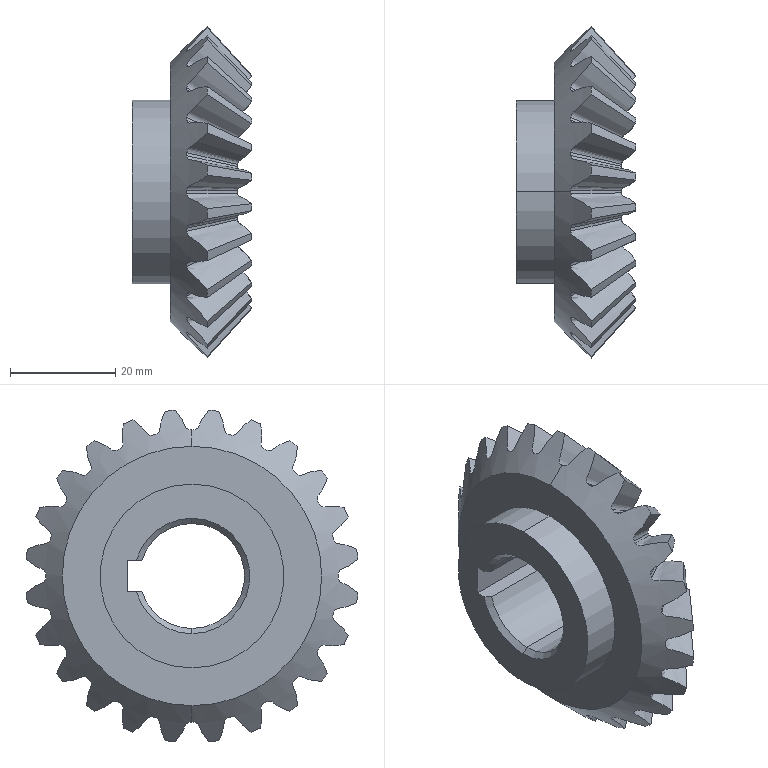Part | SolidWorks | features ICE 3, BlendCut 1, Chamfer 1, CirPattern 1, RefAxis 1, Revolution 1 | 1 solid | 117 faces | box 22.784 x 63.218 x 63.218 mm | volume 28481 mm3 | spline 72 | cone 31 | cylinder 7 | plane 7 | commonest cylinder face diameters 20 x3 30 x2 35 x2